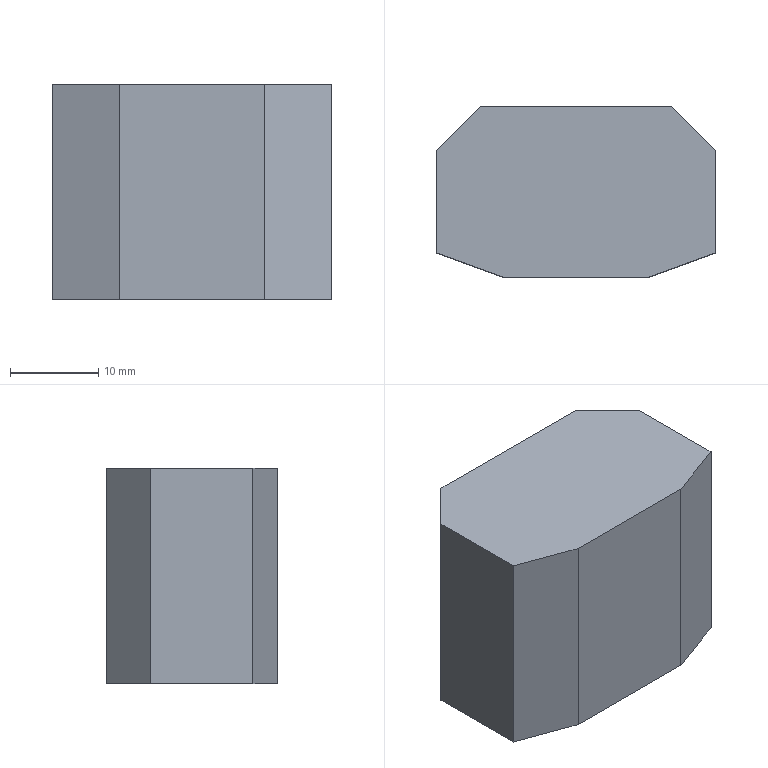Part | STEP file | 1_id1074_x_t | 1 solid | 12 faces | box 31.75 x 19.4 x 24.5 mm | volume 13473 mm3 | plane 10 | cone 1 | cylinder 1 | commonest cylinder face diameters 6.75 x1
STEP:
#1=CARTESIAN_POINT('',(0.,0.,0.));
#2=DIRECTION('',(0.,0.,1.));
#3=DIRECTION('',(1.,0.,0.));
#4=AXIS2_PLACEMENT_3D('',#1,#2,#3);
#5=CARTESIAN_POINT('',(162.471,279.927,12.25));
#6=VERTEX_POINT('',#5);
#7=CARTESIAN_POINT('',(169.221,279.927,12.25));
#8=VERTEX_POINT('',#7);
#9=CARTESIAN_POINT('',(165.846,279.927,12.25));
#10=DIRECTION('',(0.,1.,0.));
#11=DIRECTION('',(1.,0.,0.));
#12=AXIS2_PLACEMENT_3D('',#9,#10,#11);
#13=CIRCLE('',#12,3.375);
#14=CARTESIAN_POINT('',(165.846,278.973,12.25));
#15=DIRECTION('',(0.,1.,0.));
#16=DIRECTION('',(-1.,0.,0.));
#17=AXIS2_PLACEMENT_3D('',#14,#15,#16);
#18=CONICAL_SURFACE('',#17,1.721,1.047);
#19=CARTESIAN_POINT('',(-3.142,0.9548));
#20=DIRECTION('',(1.,0.));
#21=VECTOR('',#20,1.);
#22=LINE('',#19,#21);
#23=(GEOMETRIC_REPRESENTATION_CONTEXT(2)PARAMETRIC_REPRESENTATION_CONTEXT()REPRESENTATION_CONTEXT('',''));
#24=DEFINITIONAL_REPRESENTATION('',(#22),#23);
#25=PCURVE('',#18,#24);
#26=CARTESIAN_POINT('',(165.846,279.927,12.25));
#27=DIRECTION('',(0.,-1.,0.));
#28=DIRECTION('',(-1.,0.,0.));
#29=AXIS2_PLACEMENT_3D('',#26,#27,#28);
#30=CYLINDRICAL_SURFACE('',#29,3.375);
#31=CARTESIAN_POINT('',(9.425,0.));
#32=DIRECTION('',(-1.,0.));
#33=VECTOR('',#32,1.);
#34=LINE('',#31,#33);
#35=(GEOMETRIC_REPRESENTATION_CONTEXT(2)PARAMETRIC_REPRESENTATION_CONTEXT()REPRESENTATION_CONTEXT('',''));
#36=DEFINITIONAL_REPRESENTATION('',(#34),#35);
#37=PCURVE('',#30,#36);
#38=SURFACE_CURVE('',#13,(#25,#37),.PCURVE_S1.);
#39=EDGE_CURVE('',#6,#8,#38,.T.);
#40=ORIENTED_EDGE('',*,*,#39,.F.);
#41=CARTESIAN_POINT('',(165.846,277.979,12.25));
#42=VERTEX_POINT('',#41);
#43=CARTESIAN_POINT('',(165.846,277.979,12.25));
#44=CARTESIAN_POINT('',(162.471,279.927,12.25));
#45=B_SPLINE_CURVE_WITH_KNOTS('',1,(#43,#44),.UNSPECIFIED.,.F.,.F.,(2,2),(-1.988,1.91),.PIECEWISE_BEZIER_KNOTS.);
#46=CARTESIAN_POINT('',(0.,0.));
#47=DIRECTION('',(0.,1.));
#48=VECTOR('',#47,1.);
#49=LINE('',#46,#48);
#50=(GEOMETRIC_REPRESENTATION_CONTEXT(2)PARAMETRIC_REPRESENTATION_CONTEXT()REPRESENTATION_CONTEXT('',''));
#51=DEFINITIONAL_REPRESENTATION('',(#49),#50);
#52=PCURVE('',#18,#51);
#53=CARTESIAN_POINT('',(6.283,0.));
#54=DIRECTION('',(0.,1.));
#55=VECTOR('',#54,1.);
#56=LINE('',#53,#55);
#57=(GEOMETRIC_REPRESENTATION_CONTEXT(2)PARAMETRIC_REPRESENTATION_CONTEXT()REPRESENTATION_CONTEXT('',''));
#58=DEFINITIONAL_REPRESENTATION('',(#56),#57);
#59=PCURVE('',#18,#58);
#60=SEAM_CURVE('',#45,(#52,#59),.PCURVE_S1.);
#61=EDGE_CURVE('',#42,#6,#60,.T.);
#62=ORIENTED_EDGE('',*,*,#61,.F.);
#63=ORIENTED_EDGE('',*,*,#61,.T.);
#64=CARTESIAN_POINT('',(165.846,279.927,12.25));
#65=DIRECTION('',(0.,1.,0.));
#66=DIRECTION('',(1.,0.,0.));
#67=AXIS2_PLACEMENT_3D('',#64,#65,#66);
#68=CIRCLE('',#67,3.375);
#69=CARTESIAN_POINT('',(3.142,0.9548));
#70=DIRECTION('',(1.,0.));
#71=VECTOR('',#70,1.);
#72=LINE('',#69,#71);
#73=(GEOMETRIC_REPRESENTATION_CONTEXT(2)PARAMETRIC_REPRESENTATION_CONTEXT()REPRESENTATION_CONTEXT('',''));
#74=DEFINITIONAL_REPRESENTATION('',(#72),#73);
#75=PCURVE('',#18,#74);
#76=CARTESIAN_POINT('',(3.142,0.));
#77=DIRECTION('',(-1.,0.));
#78=VECTOR('',#77,1.);
#79=LINE('',#76,#78);
#80=(GEOMETRIC_REPRESENTATION_CONTEXT(2)PARAMETRIC_REPRESENTATION_CONTEXT()REPRESENTATION_CONTEXT('',''));
#81=DEFINITIONAL_REPRESENTATION('',(#79),#80);
#82=PCURVE('',#30,#81);
#83=SURFACE_CURVE('',#68,(#75,#82),.PCURVE_S1.);
#84=EDGE_CURVE('',#8,#6,#83,.T.);
#85=ORIENTED_EDGE('',*,*,#84,.F.);
#86=EDGE_LOOP('',(#40,#62,#63,#85));
#87=FACE_BOUND('',#86,.F.);
#88=ADVANCED_FACE('',(#87),#18,.F.);
#89=ORIENTED_EDGE('',*,*,#39,.T.);
#90=ORIENTED_EDGE('',*,*,#84,.T.);
#91=CARTESIAN_POINT('',(162.471,292.903,12.25));
#92=VERTEX_POINT('',#91);
#93=CARTESIAN_POINT('',(162.471,292.903,12.25));
#94=CARTESIAN_POINT('',(162.471,279.927,12.25));
#95=B_SPLINE_CURVE_WITH_KNOTS('',1,(#93,#94),.UNSPECIFIED.,.F.,.F.,(2,2),(-12.976,0.),.PIECEWISE_BEZIER_KNOTS.);
#96=CARTESIAN_POINT('',(0.,0.));
#97=DIRECTION('',(0.,1.));
#98=VECTOR('',#97,1.);
#99=LINE('',#96,#98);
#100=(GEOMETRIC_REPRESENTATION_CONTEXT(2)PARAMETRIC_REPRESENTATION_CONTEXT()REPRESENTATION_CONTEXT('',''));
#101=DEFINITIONAL_REPRESENTATION('',(#99),#100);
#102=PCURVE('',#30,#101);
#103=CARTESIAN_POINT('',(6.283,0.));
#104=DIRECTION('',(0.,1.));
#105=VECTOR('',#104,1.);
#106=LINE('',#103,#105);
#107=(GEOMETRIC_REPRESENTATION_CONTEXT(2)PARAMETRIC_REPRESENTATION_CONTEXT()REPRESENTATION_CONTEXT('',''));
#108=DEFINITIONAL_REPRESENTATION('',(#106),#107);
#109=PCURVE('',#30,#108);
#110=SEAM_CURVE('',#95,(#102,#109),.PCURVE_S1.);
#111=EDGE_CURVE('',#92,#6,#110,.T.);
#112=ORIENTED_EDGE('',*,*,#111,.F.);
#113=CARTESIAN_POINT('',(165.846,292.903,12.25));
#114=DIRECTION('',(0.,-1.,0.));
#115=DIRECTION('',(-1.,0.,0.));
#116=AXIS2_PLACEMENT_3D('',#113,#114,#115);
#117=CIRCLE('',#116,3.375);
#118=CARTESIAN_POINT('',(0.,-12.976));
#119=DIRECTION('',(1.,0.));
#120=VECTOR('',#119,1.);
#121=LINE('',#118,#120);
#122=(GEOMETRIC_REPRESENTATION_CONTEXT(2)PARAMETRIC_REPRESENTATION_CONTEXT()REPRESENTATION_CONTEXT('',''));
#123=DEFINITIONAL_REPRESENTATION('',(#121),#122);
#124=PCURVE('',#30,#123);
#125=CARTESIAN_POINT('',(252.785,292.903,-25.177));
#126=DIRECTION('',(0.,1.,0.));
#127=DIRECTION('',(-1.,0.,0.));
#128=AXIS2_PLACEMENT_3D('',#125,#126,#127);
#129=PLANE('',#128);
#130=CARTESIAN_POINT('',(90.314,37.427));
#131=CARTESIAN_POINT('',(90.314,31.581));
#132=CARTESIAN_POINT('',(85.252,34.504));
#133=CARTESIAN_POINT('',(80.189,37.427));
#134=CARTESIAN_POINT('',(85.252,40.35));
#135=CARTESIAN_POINT('',(90.314,43.273));
#136=CARTESIAN_POINT('',(90.314,37.427));
#137=(BOUNDED_CURVE()B_SPLINE_CURVE(2,(#130,#131,#132,#133,#134,#135,#136),.UNSPECIFIED.,.T.,.F.)B_SPLINE_CURVE_WITH_KNOTS((1,2,2,2,2,1),(-2.094,0.,2.094,4.189,6.283,8.378),.UNSPECIFIED.)CURVE()GEOMETRIC_REPRESENTATION_ITEM()RATIONAL_B_SPLINE_CURVE((1.,0.5,1.,0.5,1.,0.5,1.))REPRESENTATION_ITEM(''));
#138=(GEOMETRIC_REPRESENTATION_CONTEXT(2)PARAMETRIC_REPRESENTATION_CONTEXT()REPRESENTATION_CONTEXT('',''));
#139=DEFINITIONAL_REPRESENTATION('',(#137),#138);
#140=PCURVE('',#129,#139);
#141=SURFACE_CURVE('',#117,(#124,#140),.PCURVE_S1.);
#142=EDGE_CURVE('',#92,#92,#141,.T.);
#143=ORIENTED_EDGE('',*,*,#142,.T.);
#144=ORIENTED_EDGE('',*,*,#111,.T.);
#145=EDGE_LOOP('',(#89,#90,#112,#143,#144));
#146=FACE_BOUND('',#145,.F.);
#147=ADVANCED_FACE('',(#146),#30,.F.);
#148=CARTESIAN_POINT('',(154.971,292.903,24.5));
#149=VERTEX_POINT('',#148);
#150=CARTESIAN_POINT('',(154.971,292.903,0.));
#151=VERTEX_POINT('',#150);
#152=CARTESIAN_POINT('',(154.971,292.903,24.5));
#153=DIRECTION('',(0.,0.,-1.));
#154=VECTOR('',#153,1.);
#155=LINE('',#152,#154);
#156=CARTESIAN_POINT('',(97.814,49.677));
#157=DIRECTION('',(0.,-1.));
#158=VECTOR('',#157,1.);
#159=LINE('',#156,#158);
#160=(GEOMETRIC_REPRESENTATION_CONTEXT(2)PARAMETRIC_REPRESENTATION_CONTEXT()REPRESENTATION_CONTEXT('',''));
#161=DEFINITIONAL_REPRESENTATION('',(#159),#160);
#162=PCURVE('',#129,#161);
#163=CARTESIAN_POINT('',(149.971,287.903,0.1));
#164=DIRECTION('',(0.7071,-0.7071,0.));
#165=DIRECTION('',(0.,0.,1.));
#166=AXIS2_PLACEMENT_3D('',#163,#164,#165);
#167=PLANE('',#166);
#168=CARTESIAN_POINT('',(24.4,-7.071));
#169=DIRECTION('',(-1.,0.));
#170=VECTOR('',#169,1.);
#171=LINE('',#168,#170);
#172=(GEOMETRIC_REPRESENTATION_CONTEXT(2)PARAMETRIC_REPRESENTATION_CONTEXT()REPRESENTATION_CONTEXT('',''));
#173=DEFINITIONAL_REPRESENTATION('',(#171),#172);
#174=PCURVE('',#167,#173);
#175=SURFACE_CURVE('',#155,(#162,#174),.PCURVE_S1.);
#176=EDGE_CURVE('',#149,#151,#175,.T.);
#177=ORIENTED_EDGE('',*,*,#176,.F.);
#178=CARTESIAN_POINT('',(176.721,292.903,24.5));
#179=VERTEX_POINT('',#178);
#180=CARTESIAN_POINT('',(154.971,292.903,24.5));
#181=DIRECTION('',(1.,0.,0.));
#182=VECTOR('',#181,1.);
#183=LINE('',#180,#182);
#184=CARTESIAN_POINT('',(97.814,49.677));
#185=DIRECTION('',(-1.,0.));
#186=VECTOR('',#185,1.);
#187=LINE('',#184,#186);
#188=(GEOMETRIC_REPRESENTATION_CONTEXT(2)PARAMETRIC_REPRESENTATION_CONTEXT()REPRESENTATION_CONTEXT('',''));
#189=DEFINITIONAL_REPRESENTATION('',(#187),#188);
#190=PCURVE('',#129,#189);
#191=CARTESIAN_POINT('',(278.801,322.904,24.5));
#192=DIRECTION('',(0.,0.,1.));
#193=DIRECTION('',(-1.,0.,0.));
#194=AXIS2_PLACEMENT_3D('',#191,#192,#193);
#195=PLANE('',#194);
#196=CARTESIAN_POINT('',(123.83,30.));
#197=DIRECTION('',(-1.,0.));
#198=VECTOR('',#197,1.);
#199=LINE('',#196,#198);
#200=(GEOMETRIC_REPRESENTATION_CONTEXT(2)PARAMETRIC_REPRESENTATION_CONTEXT()REPRESENTATION_CONTEXT('',''));
#201=DEFINITIONAL_REPRESENTATION('',(#199),#200);
#202=PCURVE('',#195,#201);
#203=SURFACE_CURVE('',#183,(#190,#202),.PCURVE_S1.);
#204=EDGE_CURVE('',#149,#179,#203,.T.);
#205=ORIENTED_EDGE('',*,*,#204,.T.);
#206=CARTESIAN_POINT('',(176.721,292.903,0.));
#207=VERTEX_POINT('',#206);
#208=CARTESIAN_POINT('',(176.721,292.903,0.));
#209=DIRECTION('',(0.,0.,1.));
#210=VECTOR('',#209,1.);
#211=LINE('',#208,#210);
#212=CARTESIAN_POINT('',(76.064,25.177));
#213=DIRECTION('',(0.,1.));
#214=VECTOR('',#213,1.);
#215=LINE('',#212,#214);
#216=(GEOMETRIC_REPRESENTATION_CONTEXT(2)PARAMETRIC_REPRESENTATION_CONTEXT()REPRESENTATION_CONTEXT('',''));
#217=DEFINITIONAL_REPRESENTATION('',(#215),#216);
#218=PCURVE('',#129,#217);
#219=CARTESIAN_POINT('',(181.721,287.903,0.1));
#220=DIRECTION('',(-0.7071,-0.7071,0.));
#221=DIRECTION('',(0.7071,-0.7071,0.));
#222=AXIS2_PLACEMENT_3D('',#219,#220,#221);
#223=PLANE('',#222);
#224=CARTESIAN_POINT('',(-7.071,-0.1));
#225=DIRECTION('',(0.,1.));
#226=VECTOR('',#225,1.);
#227=LINE('',#224,#226);
#228=(GEOMETRIC_REPRESENTATION_CONTEXT(2)PARAMETRIC_REPRESENTATION_CONTEXT()REPRESENTATION_CONTEXT('',''));
#229=DEFINITIONAL_REPRESENTATION('',(#227),#228);
#230=PCURVE('',#223,#229);
#231=SURFACE_CURVE('',#211,(#218,#230),.PCURVE_S1.);
#232=EDGE_CURVE('',#207,#179,#231,.T.);
#233=ORIENTED_EDGE('',*,*,#232,.F.);
#234=CARTESIAN_POINT('',(154.971,292.903,0.));
#235=DIRECTION('',(1.,0.,0.));
#236=VECTOR('',#235,1.);
#237=LINE('',#234,#236);
#238=CARTESIAN_POINT('',(97.814,25.177));
#239=DIRECTION('',(-1.,0.));
#240=VECTOR('',#239,1.);
#241=LINE('',#238,#240);
#242=(GEOMETRIC_REPRESENTATION_CONTEXT(2)PARAMETRIC_REPRESENTATION_CONTEXT()REPRESENTATION_CONTEXT('',''));
#243=DEFINITIONAL_REPRESENTATION('',(#241),#242);
#244=PCURVE('',#129,#243);
#245=CARTESIAN_POINT('',(298.801,325.227,0.));
#246=DIRECTION('',(0.,0.,-1.));
#247=DIRECTION('',(0.,1.,0.));
#248=AXIS2_PLACEMENT_3D('',#245,#246,#247);
#249=PLANE('',#248);
#250=CARTESIAN_POINT('',(-32.324,-143.83));
#251=DIRECTION('',(0.,1.));
#252=VECTOR('',#251,1.);
#253=LINE('',#250,#252);
#254=(GEOMETRIC_REPRESENTATION_CONTEXT(2)PARAMETRIC_REPRESENTATION_CONTEXT()REPRESENTATION_CONTEXT('',''));
#255=DEFINITIONAL_REPRESENTATION('',(#253),#254);
#256=PCURVE('',#249,#255);
#257=SURFACE_CURVE('',#237,(#244,#256),.PCURVE_S1.);
#258=EDGE_CURVE('',#151,#207,#257,.T.);
#259=ORIENTED_EDGE('',*,*,#258,.F.);
#260=EDGE_LOOP('',(#177,#205,#233,#259));
#261=FACE_BOUND('',#260,.T.);
#262=ORIENTED_EDGE('',*,*,#142,.T.);
#263=EDGE_LOOP('',(#262));
#264=FACE_BOUND('',#263,.T.);
#265=ADVANCED_FACE('',(#261,#264),#129,.T.);
#266=CARTESIAN_POINT('',(149.971,287.903,0.));
#267=VERTEX_POINT('',#266);
#268=CARTESIAN_POINT('',(149.971,287.903,0.));
#269=DIRECTION('',(0.7071,0.7071,0.));
#270=VECTOR('',#269,1.);
#271=LINE('',#268,#270);
#272=CARTESIAN_POINT('',(-37.324,-148.83));
#273=DIRECTION('',(0.7071,0.7071));
#274=VECTOR('',#273,1.);
#275=LINE('',#272,#274);
#276=(GEOMETRIC_REPRESENTATION_CONTEXT(2)PARAMETRIC_REPRESENTATION_CONTEXT()REPRESENTATION_CONTEXT('',''));
#277=DEFINITIONAL_REPRESENTATION('',(#275),#276);
#278=PCURVE('',#249,#277);
#279=CARTESIAN_POINT('',(-0.1,0.));
#280=DIRECTION('',(0.,-1.));
#281=VECTOR('',#280,1.);
#282=LINE('',#279,#281);
#283=(GEOMETRIC_REPRESENTATION_CONTEXT(2)PARAMETRIC_REPRESENTATION_CONTEXT()REPRESENTATION_CONTEXT('',''));
#284=DEFINITIONAL_REPRESENTATION('',(#282),#283);
#285=PCURVE('',#167,#284);
#286=SURFACE_CURVE('',#271,(#278,#285),.PCURVE_S1.);
#287=EDGE_CURVE('',#267,#151,#286,.T.);
#288=ORIENTED_EDGE('',*,*,#287,.T.);
#289=ORIENTED_EDGE('',*,*,#258,.T.);
#290=CARTESIAN_POINT('',(181.721,287.903,0.));
#291=VERTEX_POINT('',#290);
#292=CARTESIAN_POINT('',(176.721,292.903,0.));
#293=DIRECTION('',(0.7071,-0.7071,0.));
#294=VECTOR('',#293,1.);
#295=LINE('',#292,#294);
#296=CARTESIAN_POINT('',(-32.324,-122.08));
#297=DIRECTION('',(-0.7071,0.7071));
#298=VECTOR('',#297,1.);
#299=LINE('',#296,#298);
#300=(GEOMETRIC_REPRESENTATION_CONTEXT(2)PARAMETRIC_REPRESENTATION_CONTEXT()REPRESENTATION_CONTEXT('',''));
#301=DEFINITIONAL_REPRESENTATION('',(#299),#300);
#302=PCURVE('',#249,#301);
#303=CARTESIAN_POINT('',(-7.071,-0.1));
#304=DIRECTION('',(1.,0.));
#305=VECTOR('',#304,1.);
#306=LINE('',#303,#305);
#307=(GEOMETRIC_REPRESENTATION_CONTEXT(2)PARAMETRIC_REPRESENTATION_CONTEXT()REPRESENTATION_CONTEXT('',''));
#308=DEFINITIONAL_REPRESENTATION('',(#306),#307);
#309=PCURVE('',#223,#308);
#310=SURFACE_CURVE('',#295,(#302,#309),.PCURVE_S1.);
#311=EDGE_CURVE('',#207,#291,#310,.T.);
#312=ORIENTED_EDGE('',*,*,#311,.T.);
#313=CARTESIAN_POINT('',(181.721,276.277,0.));
#314=VERTEX_POINT('',#313);
#315=CARTESIAN_POINT('',(181.721,276.277,0.));
#316=DIRECTION('',(0.,1.,0.));
#317=VECTOR('',#316,1.);
#318=LINE('',#315,#317);
#319=CARTESIAN_POINT('',(-48.951,-117.08));
#320=DIRECTION('',(1.,0.));
#321=VECTOR('',#320,1.);
#322=LINE('',#319,#321);
#323=(GEOMETRIC_REPRESENTATION_CONTEXT(2)PARAMETRIC_REPRESENTATION_CONTEXT()REPRESENTATION_CONTEXT('',''));
#324=DEFINITIONAL_REPRESENTATION('',(#322),#323);
#325=PCURVE('',#249,#324);
#326=CARTESIAN_POINT('',(181.721,299.827,0.1));
#327=DIRECTION('',(1.,0.,0.));
#328=DIRECTION('',(0.,-1.,0.));
#329=AXIS2_PLACEMENT_3D('',#326,#327,#328);
#330=PLANE('',#329);
#331=CARTESIAN_POINT('',(23.551,0.1));
#332=DIRECTION('',(-1.,0.));
#333=VECTOR('',#332,1.);
#334=LINE('',#331,#333);
#335=(GEOMETRIC_REPRESENTATION_CONTEXT(2)PARAMETRIC_REPRESENTATION_CONTEXT()REPRESENTATION_CONTEXT('',''));
#336=DEFINITIONAL_REPRESENTATION('',(#334),#335);
#337=PCURVE('',#330,#336);
#338=SURFACE_CURVE('',#318,(#325,#337),.PCURVE_S1.);
#339=EDGE_CURVE('',#314,#291,#338,.T.);
#340=ORIENTED_EDGE('',*,*,#339,.F.);
#341=CARTESIAN_POINT('',(174.101,273.503,0.));
#342=VERTEX_POINT('',#341);
#343=CARTESIAN_POINT('',(181.721,276.277,0.));
#344=DIRECTION('',(-0.9397,-0.342,0.));
#345=VECTOR('',#344,1.);
#346=LINE('',#343,#345);
#347=CARTESIAN_POINT('',(-48.951,-117.08));
#348=DIRECTION('',(-0.342,-0.9397));
#349=VECTOR('',#348,1.);
#350=LINE('',#347,#349);
#351=(GEOMETRIC_REPRESENTATION_CONTEXT(2)PARAMETRIC_REPRESENTATION_CONTEXT()REPRESENTATION_CONTEXT('',''));
#352=DEFINITIONAL_REPRESENTATION('',(#350),#351);
#353=PCURVE('',#249,#352);
#354=CARTESIAN_POINT('',(181.721,276.277,0.1));
#355=DIRECTION('',(0.342,-0.9397,0.));
#356=DIRECTION('',(0.,0.,1.));
#357=AXIS2_PLACEMENT_3D('',#354,#355,#356);
#358=PLANE('',#357);
#359=CARTESIAN_POINT('',(-0.1,0.));
#360=DIRECTION('',(0.,1.));
#361=VECTOR('',#360,1.);
#362=LINE('',#359,#361);
#363=(GEOMETRIC_REPRESENTATION_CONTEXT(2)PARAMETRIC_REPRESENTATION_CONTEXT()REPRESENTATION_CONTEXT('',''));
#364=DEFINITIONAL_REPRESENTATION('',(#362),#363);
#365=PCURVE('',#358,#364);
#366=SURFACE_CURVE('',#346,(#353,#365),.PCURVE_S1.);
#367=EDGE_CURVE('',#314,#342,#366,.T.);
#368=ORIENTED_EDGE('',*,*,#367,.T.);
#369=CARTESIAN_POINT('',(157.591,273.503,0.));
#370=VERTEX_POINT('',#369);
#371=CARTESIAN_POINT('',(157.591,273.503,0.));
#372=DIRECTION('',(1.,0.,0.));
#373=VECTOR('',#372,1.);
#374=LINE('',#371,#373);
#375=CARTESIAN_POINT('',(-51.724,-141.21));
#376=DIRECTION('',(0.,1.));
#377=VECTOR('',#376,1.);
#378=LINE('',#375,#377);
#379=(GEOMETRIC_REPRESENTATION_CONTEXT(2)PARAMETRIC_REPRESENTATION_CONTEXT()REPRESENTATION_CONTEXT('',''));
#380=DEFINITIONAL_REPRESENTATION('',(#378),#379);
#381=PCURVE('',#249,#380);
#382=CARTESIAN_POINT('',(174.101,273.503,0.1));
#383=DIRECTION('',(0.,-1.,0.));
#384=DIRECTION('',(0.,0.,1.));
#385=AXIS2_PLACEMENT_3D('',#382,#383,#384);
#386=PLANE('',#385);
#387=CARTESIAN_POINT('',(-0.1,16.51));
#388=DIRECTION('',(0.,-1.));
#389=VECTOR('',#388,1.);
#390=LINE('',#387,#389);
#391=(GEOMETRIC_REPRESENTATION_CONTEXT(2)PARAMETRIC_REPRESENTATION_CONTEXT()REPRESENTATION_CONTEXT('',''));
#392=DEFINITIONAL_REPRESENTATION('',(#390),#391);
#393=PCURVE('',#386,#392);
#394=SURFACE_CURVE('',#374,(#381,#393),.PCURVE_S1.);
#395=EDGE_CURVE('',#370,#342,#394,.T.);
#396=ORIENTED_EDGE('',*,*,#395,.F.);
#397=CARTESIAN_POINT('',(149.971,276.277,0.));
#398=VERTEX_POINT('',#397);
#399=CARTESIAN_POINT('',(157.591,273.503,0.));
#400=DIRECTION('',(-0.9397,0.342,0.));
#401=VECTOR('',#400,1.);
#402=LINE('',#399,#401);
#403=CARTESIAN_POINT('',(-51.724,-141.21));
#404=DIRECTION('',(0.342,-0.9397));
#405=VECTOR('',#404,1.);
#406=LINE('',#403,#405);
#407=(GEOMETRIC_REPRESENTATION_CONTEXT(2)PARAMETRIC_REPRESENTATION_CONTEXT()REPRESENTATION_CONTEXT('',''));
#408=DEFINITIONAL_REPRESENTATION('',(#406),#407);
#409=PCURVE('',#249,#408);
#410=CARTESIAN_POINT('',(157.591,273.503,0.1));
#411=DIRECTION('',(-0.342,-0.9397,0.));
#412=DIRECTION('',(0.9397,-0.342,0.));
#413=AXIS2_PLACEMENT_3D('',#410,#411,#412);
#414=PLANE('',#413);
#415=CARTESIAN_POINT('',(0.,-0.1));
#416=DIRECTION('',(-1.,0.));
#417=VECTOR('',#416,1.);
#418=LINE('',#415,#417);
#419=(GEOMETRIC_REPRESENTATION_CONTEXT(2)PARAMETRIC_REPRESENTATION_CONTEXT()REPRESENTATION_CONTEXT('',''));
#420=DEFINITIONAL_REPRESENTATION('',(#418),#419);
#421=PCURVE('',#414,#420);
#422=SURFACE_CURVE('',#402,(#409,#421),.PCURVE_S1.);
#423=EDGE_CURVE('',#370,#398,#422,.T.);
#424=ORIENTED_EDGE('',*,*,#423,.T.);
#425=CARTESIAN_POINT('',(149.971,287.903,0.));
#426=DIRECTION('',(0.,-1.,0.));
#427=VECTOR('',#426,1.);
#428=LINE('',#425,#427);
#429=CARTESIAN_POINT('',(-37.324,-148.83));
#430=DIRECTION('',(-1.,0.));
#431=VECTOR('',#430,1.);
#432=LINE('',#429,#431);
#433=(GEOMETRIC_REPRESENTATION_CONTEXT(2)PARAMETRIC_REPRESENTATION_CONTEXT()REPRESENTATION_CONTEXT('',''));
#434=DEFINITIONAL_REPRESENTATION('',(#432),#433);
#435=PCURVE('',#249,#434);
#436=CARTESIAN_POINT('',(149.971,275.677,0.1));
#437=DIRECTION('',(-1.,0.,0.));
#438=DIRECTION('',(0.,-1.,0.));
#439=AXIS2_PLACEMENT_3D('',#436,#437,#438);
#440=PLANE('',#439);
#441=CARTESIAN_POINT('',(-12.227,-0.1));
#442=DIRECTION('',(1.,0.));
#443=VECTOR('',#442,1.);
#444=LINE('',#441,#443);
#445=(GEOMETRIC_REPRESENTATION_CONTEXT(2)PARAMETRIC_REPRESENTATION_CONTEXT()REPRESENTATION_CONTEXT('',''));
#446=DEFINITIONAL_REPRESENTATION('',(#444),#445);
#447=PCURVE('',#440,#446);
#448=SURFACE_CURVE('',#428,(#435,#447),.PCURVE_S1.);
#449=EDGE_CURVE('',#267,#398,#448,.T.);
#450=ORIENTED_EDGE('',*,*,#449,.F.);
#451=EDGE_LOOP('',(#288,#289,#312,#340,#368,#396,#424,#450));
#452=FACE_BOUND('',#451,.T.);
#453=ADVANCED_FACE('',(#452),#249,.T.);
#454=CARTESIAN_POINT('',(149.971,287.903,24.5));
#455=VERTEX_POINT('',#454);
#456=CARTESIAN_POINT('',(149.971,287.903,0.));
#457=DIRECTION('',(0.,0.,1.));
#458=VECTOR('',#457,1.);
#459=LINE('',#456,#458);
#460=CARTESIAN_POINT('',(-12.227,-0.1));
#461=DIRECTION('',(0.,1.));
#462=VECTOR('',#461,1.);
#463=LINE('',#460,#462);
#464=(GEOMETRIC_REPRESENTATION_CONTEXT(2)PARAMETRIC_REPRESENTATION_CONTEXT()REPRESENTATION_CONTEXT('',''));
#465=DEFINITIONAL_REPRESENTATION('',(#463),#464);
#466=PCURVE('',#440,#465);
#467=CARTESIAN_POINT('',(-0.1,0.));
#468=DIRECTION('',(1.,0.));
#469=VECTOR('',#468,1.);
#470=LINE('',#467,#469);
#471=(GEOMETRIC_REPRESENTATION_CONTEXT(2)PARAMETRIC_REPRESENTATION_CONTEXT()REPRESENTATION_CONTEXT('',''));
#472=DEFINITIONAL_REPRESENTATION('',(#470),#471);
#473=PCURVE('',#167,#472);
#474=SURFACE_CURVE('',#459,(#466,#473),.PCURVE_S1.);
#475=EDGE_CURVE('',#267,#455,#474,.T.);
#476=ORIENTED_EDGE('',*,*,#475,.F.);
#477=ORIENTED_EDGE('',*,*,#449,.T.);
#478=CARTESIAN_POINT('',(149.971,276.277,24.5));
#479=VERTEX_POINT('',#478);
#480=CARTESIAN_POINT('',(149.971,276.277,24.5));
#481=DIRECTION('',(0.,0.,-1.));
#482=VECTOR('',#481,1.);
#483=LINE('',#480,#482);
#484=CARTESIAN_POINT('',(-0.6,24.4));
#485=DIRECTION('',(0.,-1.));
#486=VECTOR('',#485,1.);
#487=LINE('',#484,#486);
#488=(GEOMETRIC_REPRESENTATION_CONTEXT(2)PARAMETRIC_REPRESENTATION_CONTEXT()REPRESENTATION_CONTEXT('',''));
#489=DEFINITIONAL_REPRESENTATION('',(#487),#488);
#490=PCURVE('',#440,#489);
#491=CARTESIAN_POINT('',(-8.109,24.4));
#492=DIRECTION('',(0.,-1.));
#493=VECTOR('',#492,1.);
#494=LINE('',#491,#493);
#495=(GEOMETRIC_REPRESENTATION_CONTEXT(2)PARAMETRIC_REPRESENTATION_CONTEXT()REPRESENTATION_CONTEXT('',''));
#496=DEFINITIONAL_REPRESENTATION('',(#494),#495);
#497=PCURVE('',#414,#496);
#498=SURFACE_CURVE('',#483,(#490,#497),.PCURVE_S1.);
#499=EDGE_CURVE('',#479,#398,#498,.T.);
#500=ORIENTED_EDGE('',*,*,#499,.F.);
#501=CARTESIAN_POINT('',(149.971,287.903,24.5));
#502=DIRECTION('',(0.,-1.,0.));
#503=VECTOR('',#502,1.);
#504=LINE('',#501,#503);
#505=CARTESIAN_POINT('',(-12.227,24.4));
#506=DIRECTION('',(1.,0.));
#507=VECTOR('',#506,1.);
#508=LINE('',#505,#507);
#509=(GEOMETRIC_REPRESENTATION_CONTEXT(2)PARAMETRIC_REPRESENTATION_CONTEXT()REPRESENTATION_CONTEXT('',''));
#510=DEFINITIONAL_REPRESENTATION('',(#508),#509);
#511=PCURVE('',#440,#510);
#512=CARTESIAN_POINT('',(128.83,35.));
#513=DIRECTION('',(0.,1.));
#514=VECTOR('',#513,1.);
#515=LINE('',#512,#514);
#516=(GEOMETRIC_REPRESENTATION_CONTEXT(2)PARAMETRIC_REPRESENTATION_CONTEXT()REPRESENTATION_CONTEXT('',''));
#517=DEFINITIONAL_REPRESENTATION('',(#515),#516);
#518=PCURVE('',#195,#517);
#519=SURFACE_CURVE('',#504,(#511,#518),.PCURVE_S1.);
#520=EDGE_CURVE('',#455,#479,#519,.T.);
#521=ORIENTED_EDGE('',*,*,#520,.F.);
#522=EDGE_LOOP('',(#476,#477,#500,#521));
#523=FACE_BOUND('',#522,.T.);
#524=ADVANCED_FACE('',(#523),#440,.T.);
#525=CARTESIAN_POINT('',(154.971,292.903,24.5));
#526=DIRECTION('',(-0.7071,-0.7071,0.));
#527=VECTOR('',#526,1.);
#528=LINE('',#525,#527);
#529=CARTESIAN_POINT('',(123.83,30.));
#530=DIRECTION('',(0.7071,0.7071));
#531=VECTOR('',#530,1.);
#532=LINE('',#529,#531);
#533=(GEOMETRIC_REPRESENTATION_CONTEXT(2)PARAMETRIC_REPRESENTATION_CONTEXT()REPRESENTATION_CONTEXT('',''));
#534=DEFINITIONAL_REPRESENTATION('',(#532),#533);
#535=PCURVE('',#195,#534);
#536=CARTESIAN_POINT('',(24.4,-7.071));
#537=DIRECTION('',(0.,1.));
#538=VECTOR('',#537,1.);
#539=LINE('',#536,#538);
#540=(GEOMETRIC_REPRESENTATION_CONTEXT(2)PARAMETRIC_REPRESENTATION_CONTEXT()REPRESENTATION_CONTEXT('',''));
#541=DEFINITIONAL_REPRESENTATION('',(#539),#540);
#542=PCURVE('',#167,#541);
#543=SURFACE_CURVE('',#528,(#535,#542),.PCURVE_S1.);
#544=EDGE_CURVE('',#149,#455,#543,.T.);
#545=ORIENTED_EDGE('',*,*,#544,.T.);
#546=ORIENTED_EDGE('',*,*,#520,.T.);
#547=CARTESIAN_POINT('',(157.591,273.503,24.5));
#548=VERTEX_POINT('',#547);
#549=CARTESIAN_POINT('',(149.971,276.277,24.5));
#550=DIRECTION('',(0.9397,-0.342,0.));
#551=VECTOR('',#550,1.);
#552=LINE('',#549,#551);
#553=CARTESIAN_POINT('',(128.83,46.627));
#554=DIRECTION('',(-0.9397,0.342));
#555=VECTOR('',#554,1.);
#556=LINE('',#553,#555);
#557=(GEOMETRIC_REPRESENTATION_CONTEXT(2)PARAMETRIC_REPRESENTATION_CONTEXT()REPRESENTATION_CONTEXT('',''));
#558=DEFINITIONAL_REPRESENTATION('',(#556),#557);
#559=PCURVE('',#195,#558);
#560=CARTESIAN_POINT('',(-8.109,24.4));
#561=DIRECTION('',(1.,0.));
#562=VECTOR('',#561,1.);
#563=LINE('',#560,#562);
#564=(GEOMETRIC_REPRESENTATION_CONTEXT(2)PARAMETRIC_REPRESENTATION_CONTEXT()REPRESENTATION_CONTEXT('',''));
#565=DEFINITIONAL_REPRESENTATION('',(#563),#564);
#566=PCURVE('',#414,#565);
#567=SURFACE_CURVE('',#552,(#559,#566),.PCURVE_S1.);
#568=EDGE_CURVE('',#479,#548,#567,.T.);
#569=ORIENTED_EDGE('',*,*,#568,.T.);
#570=CARTESIAN_POINT('',(174.101,273.503,24.5));
#571=VERTEX_POINT('',#570);
#572=CARTESIAN_POINT('',(157.591,273.503,24.5));
#573=DIRECTION('',(1.,0.,0.));
#574=VECTOR('',#573,1.);
#575=LINE('',#572,#574);
#576=CARTESIAN_POINT('',(121.21,49.4));
#577=DIRECTION('',(-1.,0.));
#578=VECTOR('',#577,1.);
#579=LINE('',#576,#578);
#580=(GEOMETRIC_REPRESENTATION_CONTEXT(2)PARAMETRIC_REPRESENTATION_CONTEXT()REPRESENTATION_CONTEXT('',''));
#581=DEFINITIONAL_REPRESENTATION('',(#579),#580);
#582=PCURVE('',#195,#581);
#583=CARTESIAN_POINT('',(24.4,16.51));
#584=DIRECTION('',(0.,-1.));
#585=VECTOR('',#584,1.);
#586=LINE('',#583,#585);
#587=(GEOMETRIC_REPRESENTATION_CONTEXT(2)PARAMETRIC_REPRESENTATION_CONTEXT()REPRESENTATION_CONTEXT('',''));
#588=DEFINITIONAL_REPRESENTATION('',(#586),#587);
#589=PCURVE('',#386,#588);
#590=SURFACE_CURVE('',#575,(#582,#589),.PCURVE_S1.);
#591=EDGE_CURVE('',#548,#571,#590,.T.);
#592=ORIENTED_EDGE('',*,*,#591,.T.);
#593=CARTESIAN_POINT('',(181.721,276.277,24.5));
#594=VERTEX_POINT('',#593);
#595=CARTESIAN_POINT('',(174.101,273.503,24.5));
#596=DIRECTION('',(0.9397,0.342,0.));
#597=VECTOR('',#596,1.);
#598=LINE('',#595,#597);
#599=CARTESIAN_POINT('',(104.7,49.4));
#600=DIRECTION('',(-0.9397,-0.342));
#601=VECTOR('',#600,1.);
#602=LINE('',#599,#601);
#603=(GEOMETRIC_REPRESENTATION_CONTEXT(2)PARAMETRIC_REPRESENTATION_CONTEXT()REPRESENTATION_CONTEXT('',''));
#604=DEFINITIONAL_REPRESENTATION('',(#602),#603);
#605=PCURVE('',#195,#604);
#606=CARTESIAN_POINT('',(24.4,8.109));
#607=DIRECTION('',(0.,-1.));
#608=VECTOR('',#607,1.);
#609=LINE('',#606,#608);
#610=(GEOMETRIC_REPRESENTATION_CONTEXT(2)PARAMETRIC_REPRESENTATION_CONTEXT()REPRESENTATION_CONTEXT('',''));
#611=DEFINITIONAL_REPRESENTATION('',(#609),#610);
#612=PCURVE('',#358,#611);
#613=SURFACE_CURVE('',#598,(#605,#612),.PCURVE_S1.);
#614=EDGE_CURVE('',#571,#594,#613,.T.);
#615=ORIENTED_EDGE('',*,*,#614,.T.);
#616=CARTESIAN_POINT('',(181.721,287.903,24.5));
#617=VERTEX_POINT('',#616);
#618=CARTESIAN_POINT('',(181.721,276.277,24.5));
#619=DIRECTION('',(0.,1.,0.));
#620=VECTOR('',#619,1.);
#621=LINE('',#618,#620);
#622=CARTESIAN_POINT('',(97.08,46.627));
#623=DIRECTION('',(0.,-1.));
#624=VECTOR('',#623,1.);
#625=LINE('',#622,#624);
#626=(GEOMETRIC_REPRESENTATION_CONTEXT(2)PARAMETRIC_REPRESENTATION_CONTEXT()REPRESENTATION_CONTEXT('',''));
#627=DEFINITIONAL_REPRESENTATION('',(#625),#626);
#628=PCURVE('',#195,#627);
#629=CARTESIAN_POINT('',(23.551,-24.4));
#630=DIRECTION('',(-1.,0.));
#631=VECTOR('',#630,1.);
#632=LINE('',#629,#631);
#633=(GEOMETRIC_REPRESENTATION_CONTEXT(2)PARAMETRIC_REPRESENTATION_CONTEXT()REPRESENTATION_CONTEXT('',''));
#634=DEFINITIONAL_REPRESENTATION('',(#632),#633);
#635=PCURVE('',#330,#634);
#636=SURFACE_CURVE('',#621,(#628,#635),.PCURVE_S1.);
#637=EDGE_CURVE('',#594,#617,#636,.T.);
#638=ORIENTED_EDGE('',*,*,#637,.T.);
#639=CARTESIAN_POINT('',(181.721,287.903,24.5));
#640=DIRECTION('',(-0.7071,0.7071,0.));
#641=VECTOR('',#640,1.);
#642=LINE('',#639,#641);
#643=CARTESIAN_POINT('',(97.08,35.));
#644=DIRECTION('',(0.7071,-0.7071));
#645=VECTOR('',#644,1.);
#646=LINE('',#643,#645);
#647=(GEOMETRIC_REPRESENTATION_CONTEXT(2)PARAMETRIC_REPRESENTATION_CONTEXT()REPRESENTATION_CONTEXT('',''));
#648=DEFINITIONAL_REPRESENTATION('',(#646),#647);
#649=PCURVE('',#195,#648);
#650=CARTESIAN_POINT('',(0.,24.4));
#651=DIRECTION('',(-1.,0.));
#652=VECTOR('',#651,1.);
#653=LINE('',#650,#652);
#654=(GEOMETRIC_REPRESENTATION_CONTEXT(2)PARAMETRIC_REPRESENTATION_CONTEXT()REPRESENTATION_CONTEXT('',''));
#655=DEFINITIONAL_REPRESENTATION('',(#653),#654);
#656=PCURVE('',#223,#655);
#657=SURFACE_CURVE('',#642,(#649,#656),.PCURVE_S1.);
#658=EDGE_CURVE('',#617,#179,#657,.T.);
#659=ORIENTED_EDGE('',*,*,#658,.T.);
#660=ORIENTED_EDGE('',*,*,#204,.F.);
#661=EDGE_LOOP('',(#545,#546,#569,#592,#615,#638,#659,#660));
#662=FACE_BOUND('',#661,.T.);
#663=ADVANCED_FACE('',(#662),#195,.T.);
#664=ORIENTED_EDGE('',*,*,#232,.T.);
#665=ORIENTED_EDGE('',*,*,#658,.F.);
#666=CARTESIAN_POINT('',(181.721,287.903,24.5));
#667=DIRECTION('',(0.,0.,-1.));
#668=VECTOR('',#667,1.);
#669=LINE('',#666,#668);
#670=CARTESIAN_POINT('',(0.,24.4));
#671=DIRECTION('',(0.,-1.));
#672=VECTOR('',#671,1.);
#673=LINE('',#670,#672);
#674=(GEOMETRIC_REPRESENTATION_CONTEXT(2)PARAMETRIC_REPRESENTATION_CONTEXT()REPRESENTATION_CONTEXT('',''));
#675=DEFINITIONAL_REPRESENTATION('',(#673),#674);
#676=PCURVE('',#223,#675);
#677=CARTESIAN_POINT('',(11.924,-24.4));
#678=DIRECTION('',(0.,1.));
#679=VECTOR('',#678,1.);
#680=LINE('',#677,#679);
#681=(GEOMETRIC_REPRESENTATION_CONTEXT(2)PARAMETRIC_REPRESENTATION_CONTEXT()REPRESENTATION_CONTEXT('',''));
#682=DEFINITIONAL_REPRESENTATION('',(#680),#681);
#683=PCURVE('',#330,#682);
#684=SURFACE_CURVE('',#669,(#676,#683),.PCURVE_S1.);
#685=EDGE_CURVE('',#617,#291,#684,.T.);
#686=ORIENTED_EDGE('',*,*,#685,.T.);
#687=ORIENTED_EDGE('',*,*,#311,.F.);
#688=EDGE_LOOP('',(#664,#665,#686,#687));
#689=FACE_BOUND('',#688,.T.);
#690=ADVANCED_FACE('',(#689),#223,.F.);
#691=ORIENTED_EDGE('',*,*,#685,.F.);
#692=ORIENTED_EDGE('',*,*,#637,.F.);
#693=CARTESIAN_POINT('',(181.721,276.277,24.5));
#694=DIRECTION('',(0.,0.,-1.));
#695=VECTOR('',#694,1.);
#696=LINE('',#693,#695);
#697=CARTESIAN_POINT('',(23.551,-24.4));
#698=DIRECTION('',(0.,1.));
#699=VECTOR('',#698,1.);
#700=LINE('',#697,#699);
#701=(GEOMETRIC_REPRESENTATION_CONTEXT(2)PARAMETRIC_REPRESENTATION_CONTEXT()REPRESENTATION_CONTEXT('',''));
#702=DEFINITIONAL_REPRESENTATION('',(#700),#701);
#703=PCURVE('',#330,#702);
#704=CARTESIAN_POINT('',(24.4,0.));
#705=DIRECTION('',(-1.,0.));
#706=VECTOR('',#705,1.);
#707=LINE('',#704,#706);
#708=(GEOMETRIC_REPRESENTATION_CONTEXT(2)PARAMETRIC_REPRESENTATION_CONTEXT()REPRESENTATION_CONTEXT('',''));
#709=DEFINITIONAL_REPRESENTATION('',(#707),#708);
#710=PCURVE('',#358,#709);
#711=SURFACE_CURVE('',#696,(#703,#710),.PCURVE_S1.);
#712=EDGE_CURVE('',#594,#314,#711,.T.);
#713=ORIENTED_EDGE('',*,*,#712,.T.);
#714=ORIENTED_EDGE('',*,*,#339,.T.);
#715=EDGE_LOOP('',(#691,#692,#713,#714));
#716=FACE_BOUND('',#715,.T.);
#717=ADVANCED_FACE('',(#716),#330,.T.);
#718=CARTESIAN_POINT('',(174.101,273.503,24.5));
#719=DIRECTION('',(0.,0.,-1.));
#720=VECTOR('',#719,1.);
#721=LINE('',#718,#720);
#722=CARTESIAN_POINT('',(24.4,8.109));
#723=DIRECTION('',(-1.,0.));
#724=VECTOR('',#723,1.);
#725=LINE('',#722,#724);
#726=(GEOMETRIC_REPRESENTATION_CONTEXT(2)PARAMETRIC_REPRESENTATION_CONTEXT()REPRESENTATION_CONTEXT('',''));
#727=DEFINITIONAL_REPRESENTATION('',(#725),#726);
#728=PCURVE('',#358,#727);
#729=CARTESIAN_POINT('',(24.4,0.));
#730=DIRECTION('',(-1.,0.));
#731=VECTOR('',#730,1.);
#732=LINE('',#729,#731);
#733=(GEOMETRIC_REPRESENTATION_CONTEXT(2)PARAMETRIC_REPRESENTATION_CONTEXT()REPRESENTATION_CONTEXT('',''));
#734=DEFINITIONAL_REPRESENTATION('',(#732),#733);
#735=PCURVE('',#386,#734);
#736=SURFACE_CURVE('',#721,(#728,#735),.PCURVE_S1.);
#737=EDGE_CURVE('',#571,#342,#736,.T.);
#738=ORIENTED_EDGE('',*,*,#737,.T.);
#739=ORIENTED_EDGE('',*,*,#367,.F.);
#740=ORIENTED_EDGE('',*,*,#712,.F.);
#741=ORIENTED_EDGE('',*,*,#614,.F.);
#742=EDGE_LOOP('',(#738,#739,#740,#741));
#743=FACE_BOUND('',#742,.T.);
#744=ADVANCED_FACE('',(#743),#358,.T.);
#745=CARTESIAN_POINT('',(157.591,273.503,24.5));
#746=DIRECTION('',(0.,0.,-1.));
#747=VECTOR('',#746,1.);
#748=LINE('',#745,#747);
#749=CARTESIAN_POINT('',(24.4,16.51));
#750=DIRECTION('',(-1.,0.));
#751=VECTOR('',#750,1.);
#752=LINE('',#749,#751);
#753=(GEOMETRIC_REPRESENTATION_CONTEXT(2)PARAMETRIC_REPRESENTATION_CONTEXT()REPRESENTATION_CONTEXT('',''));
#754=DEFINITIONAL_REPRESENTATION('',(#752),#753);
#755=PCURVE('',#386,#754);
#756=CARTESIAN_POINT('',(0.,24.4));
#757=DIRECTION('',(0.,-1.));
#758=VECTOR('',#757,1.);
#759=LINE('',#756,#758);
#760=(GEOMETRIC_REPRESENTATION_CONTEXT(2)PARAMETRIC_REPRESENTATION_CONTEXT()REPRESENTATION_CONTEXT('',''));
#761=DEFINITIONAL_REPRESENTATION('',(#759),#760);
#762=PCURVE('',#414,#761);
#763=SURFACE_CURVE('',#748,(#755,#762),.PCURVE_S1.);
#764=EDGE_CURVE('',#548,#370,#763,.T.);
#765=ORIENTED_EDGE('',*,*,#764,.T.);
#766=ORIENTED_EDGE('',*,*,#395,.T.);
#767=ORIENTED_EDGE('',*,*,#737,.F.);
#768=ORIENTED_EDGE('',*,*,#591,.F.);
#769=EDGE_LOOP('',(#765,#766,#767,#768));
#770=FACE_BOUND('',#769,.T.);
#771=ADVANCED_FACE('',(#770),#386,.T.);
#772=ORIENTED_EDGE('',*,*,#499,.T.);
#773=ORIENTED_EDGE('',*,*,#423,.F.);
#774=ORIENTED_EDGE('',*,*,#764,.F.);
#775=ORIENTED_EDGE('',*,*,#568,.F.);
#776=EDGE_LOOP('',(#772,#773,#774,#775));
#777=FACE_BOUND('',#776,.T.);
#778=ADVANCED_FACE('',(#777),#414,.T.);
#779=ORIENTED_EDGE('',*,*,#176,.T.);
#780=ORIENTED_EDGE('',*,*,#287,.F.);
#781=ORIENTED_EDGE('',*,*,#475,.T.);
#782=ORIENTED_EDGE('',*,*,#544,.F.);
#783=EDGE_LOOP('',(#779,#780,#781,#782));
#784=FACE_BOUND('',#783,.T.);
#785=ADVANCED_FACE('',(#784),#167,.F.);
#786=CLOSED_SHELL('',(#88,#147,#265,#453,#524,#663,#690,#717,#744,#771,#778,#785));
#787=MANIFOLD_SOLID_BREP('',#786);
#788=(LENGTH_UNIT()NAMED_UNIT(*)SI_UNIT(.MILLI.,.METRE.));
#789=UNCERTAINTY_MEASURE_WITH_UNIT(LENGTH_MEASURE(0.000001),#788,'','');
#790=(NAMED_UNIT(*)PLANE_ANGLE_UNIT()SI_UNIT($,.RADIAN.));
#791=(NAMED_UNIT(*)SI_UNIT($,.STERADIAN.)SOLID_ANGLE_UNIT());
#792=(GEOMETRIC_REPRESENTATION_CONTEXT(3)GLOBAL_UNCERTAINTY_ASSIGNED_CONTEXT((#789))GLOBAL_UNIT_ASSIGNED_CONTEXT((#788,#790,#791))REPRESENTATION_CONTEXT('',''));
#793=ADVANCED_BREP_SHAPE_REPRESENTATION('',(#4,#787),#792);